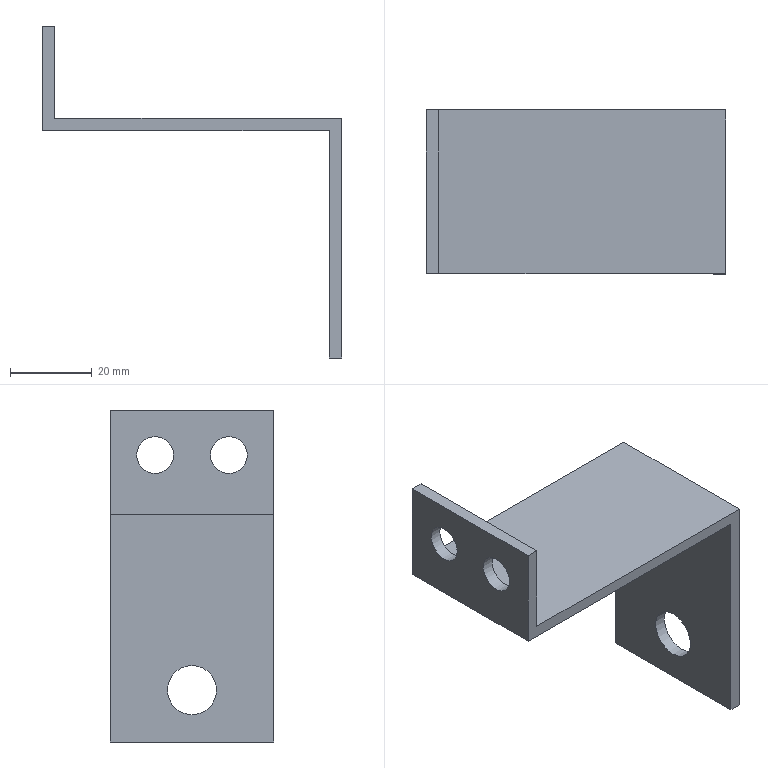Part | NX | features 1605242049 2 | 1 solid | 13 faces | box 73 x 40 x 81.051 mm | volume 17405 mm3 | plane 10 | cylinder 3 | commonest cylinder face diameters 9 x2 12 x1
STEP:
#1=CARTESIAN_POINT('',(1024.,-40.,36.449));
#2=VERTEX_POINT('',#1);
#3=CARTESIAN_POINT('',(1024.,-40.,-22.051));
#4=VERTEX_POINT('',#3);
#5=CARTESIAN_POINT('',(1024.,-40.,49.449));
#6=DIRECTION('',(0.,0.,1.));
#7=VECTOR('',#6,1000.);
#8=LINE('',#5,#7);
#9=EDGE_CURVE('',#2,#4,#8,.F.);
#10=ORIENTED_EDGE('',*,*,#9,.T.);
#11=CARTESIAN_POINT('',(1021.,-40.,-22.051));
#12=VERTEX_POINT('',#11);
#13=CARTESIAN_POINT('',(1047.,-40.,-22.051));
#14=DIRECTION('',(-1.,0.,0.));
#15=VECTOR('',#14,1000.);
#16=LINE('',#13,#15);
#17=EDGE_CURVE('',#12,#4,#16,.F.);
#18=ORIENTED_EDGE('',*,*,#17,.F.);
#19=CARTESIAN_POINT('',(1021.,-40.,33.449));
#20=VERTEX_POINT('',#19);
#21=CARTESIAN_POINT('',(1021.,-40.,6.449));
#22=DIRECTION('',(0.,0.,1.));
#23=VECTOR('',#22,1000.);
#24=LINE('',#21,#23);
#25=EDGE_CURVE('',#20,#12,#24,.F.);
#26=ORIENTED_EDGE('',*,*,#25,.F.);
#27=CARTESIAN_POINT('',(951.,-40.,33.449));
#28=VERTEX_POINT('',#27);
#29=CARTESIAN_POINT('',(973.,-40.,33.449));
#30=DIRECTION('',(-1.,0.,0.));
#31=VECTOR('',#30,1000.);
#32=LINE('',#29,#31);
#33=EDGE_CURVE('',#28,#20,#32,.F.);
#34=ORIENTED_EDGE('',*,*,#33,.F.);
#35=CARTESIAN_POINT('',(951.,-40.,59.));
#36=VERTEX_POINT('',#35);
#37=CARTESIAN_POINT('',(951.,-40.,49.449));
#38=DIRECTION('',(0.,0.,1.));
#39=VECTOR('',#38,1000.);
#40=LINE('',#37,#39);
#41=EDGE_CURVE('',#36,#28,#40,.F.);
#42=ORIENTED_EDGE('',*,*,#41,.F.);
#43=CARTESIAN_POINT('',(954.,-40.,59.));
#44=VERTEX_POINT('',#43);
#45=CARTESIAN_POINT('',(938.5,-40.,59.));
#46=DIRECTION('',(1.,0.,0.));
#47=VECTOR('',#46,1000.);
#48=LINE('',#45,#47);
#49=EDGE_CURVE('',#44,#36,#48,.F.);
#50=ORIENTED_EDGE('',*,*,#49,.F.);
#51=CARTESIAN_POINT('',(954.,-40.,36.449));
#52=VERTEX_POINT('',#51);
#53=CARTESIAN_POINT('',(954.,-40.,49.449));
#54=DIRECTION('',(0.,0.,1.));
#55=VECTOR('',#54,1000.);
#56=LINE('',#53,#55);
#57=EDGE_CURVE('',#44,#52,#56,.F.);
#58=ORIENTED_EDGE('',*,*,#57,.T.);
#59=CARTESIAN_POINT('',(973.,-40.,36.449));
#60=DIRECTION('',(-1.,0.,0.));
#61=VECTOR('',#60,1000.);
#62=LINE('',#59,#61);
#63=EDGE_CURVE('',#52,#2,#62,.F.);
#64=ORIENTED_EDGE('',*,*,#63,.T.);
#65=EDGE_LOOP('',(#10,#18,#26,#34,#42,#50,#58,#64));
#66=FACE_BOUND('',#65,.T.);
#67=CARTESIAN_POINT('',(973.,-40.,49.449));
#68=DIRECTION('',(0.,1.,0.));
#69=DIRECTION('',(1.,0.,0.));
#70=AXIS2_PLACEMENT_3D('',#67,#68,#69);
#71=PLANE('',#70);
#72=ADVANCED_FACE('',(#66),#71,.T.);
#73=CARTESIAN_POINT('',(1021.,-80.,-22.051));
#74=VERTEX_POINT('',#73);
#75=CARTESIAN_POINT('',(1021.,-80.,33.449));
#76=VERTEX_POINT('',#75);
#77=CARTESIAN_POINT('',(1021.,-80.,6.449));
#78=DIRECTION('',(0.,0.,-1.));
#79=VECTOR('',#78,1000.);
#80=LINE('',#77,#79);
#81=EDGE_CURVE('',#74,#76,#80,.F.);
#82=ORIENTED_EDGE('',*,*,#81,.F.);
#83=CARTESIAN_POINT('',(1024.,-80.,-22.051));
#84=VERTEX_POINT('',#83);
#85=CARTESIAN_POINT('',(1047.,-80.,-22.051));
#86=DIRECTION('',(1.,0.,0.));
#87=VECTOR('',#86,1000.);
#88=LINE('',#85,#87);
#89=EDGE_CURVE('',#84,#74,#88,.F.);
#90=ORIENTED_EDGE('',*,*,#89,.F.);
#91=CARTESIAN_POINT('',(1024.,-80.,36.449));
#92=VERTEX_POINT('',#91);
#93=CARTESIAN_POINT('',(1024.,-80.,49.449));
#94=DIRECTION('',(0.,0.,-1.));
#95=VECTOR('',#94,1000.);
#96=LINE('',#93,#95);
#97=EDGE_CURVE('',#84,#92,#96,.F.);
#98=ORIENTED_EDGE('',*,*,#97,.T.);
#99=CARTESIAN_POINT('',(954.,-80.,36.449));
#100=VERTEX_POINT('',#99);
#101=CARTESIAN_POINT('',(973.,-80.,36.449));
#102=DIRECTION('',(1.,0.,0.));
#103=VECTOR('',#102,1000.);
#104=LINE('',#101,#103);
#105=EDGE_CURVE('',#92,#100,#104,.F.);
#106=ORIENTED_EDGE('',*,*,#105,.T.);
#107=CARTESIAN_POINT('',(954.,-80.,59.));
#108=VERTEX_POINT('',#107);
#109=CARTESIAN_POINT('',(954.,-80.,49.449));
#110=DIRECTION('',(0.,0.,-1.));
#111=VECTOR('',#110,1000.);
#112=LINE('',#109,#111);
#113=EDGE_CURVE('',#100,#108,#112,.F.);
#114=ORIENTED_EDGE('',*,*,#113,.T.);
#115=CARTESIAN_POINT('',(951.,-80.,59.));
#116=VERTEX_POINT('',#115);
#117=CARTESIAN_POINT('',(938.5,-80.,59.));
#118=DIRECTION('',(-1.,0.,0.));
#119=VECTOR('',#118,1000.);
#120=LINE('',#117,#119);
#121=EDGE_CURVE('',#116,#108,#120,.F.);
#122=ORIENTED_EDGE('',*,*,#121,.F.);
#123=CARTESIAN_POINT('',(951.,-80.,33.449));
#124=VERTEX_POINT('',#123);
#125=CARTESIAN_POINT('',(951.,-80.,49.449));
#126=DIRECTION('',(0.,0.,-1.));
#127=VECTOR('',#126,1000.);
#128=LINE('',#125,#127);
#129=EDGE_CURVE('',#124,#116,#128,.F.);
#130=ORIENTED_EDGE('',*,*,#129,.F.);
#131=CARTESIAN_POINT('',(973.,-80.,33.449));
#132=DIRECTION('',(1.,0.,0.));
#133=VECTOR('',#132,1000.);
#134=LINE('',#131,#133);
#135=EDGE_CURVE('',#76,#124,#134,.F.);
#136=ORIENTED_EDGE('',*,*,#135,.F.);
#137=EDGE_LOOP('',(#82,#90,#98,#106,#114,#122,#130,#136));
#138=FACE_BOUND('',#137,.T.);
#139=CARTESIAN_POINT('',(973.,-80.,49.449));
#140=DIRECTION('',(0.,-1.,0.));
#141=DIRECTION('',(-1.,0.,0.));
#142=AXIS2_PLACEMENT_3D('',#139,#140,#141);
#143=PLANE('',#142);
#144=ADVANCED_FACE('',(#138),#143,.T.);
#145=CARTESIAN_POINT('',(951.,-64.5,48.));
#146=VERTEX_POINT('',#145);
#147=CARTESIAN_POINT('',(951.,-69.,48.));
#148=DIRECTION('',(1.,0.,0.));
#149=DIRECTION('',(0.,1.,0.));
#150=AXIS2_PLACEMENT_3D('',#147,#148,#149);
#151=CIRCLE('',#150,4.5);
#152=EDGE_CURVE('',#146,#146,#151,.F.);
#153=ORIENTED_EDGE('',*,*,#152,.T.);
#154=EDGE_LOOP('',(#153));
#155=FACE_BOUND('',#154,.T.);
#156=CARTESIAN_POINT('',(954.,-64.5,48.));
#157=VERTEX_POINT('',#156);
#158=CARTESIAN_POINT('',(954.,-69.,48.));
#159=DIRECTION('',(1.,0.,0.));
#160=DIRECTION('',(0.,1.,0.));
#161=AXIS2_PLACEMENT_3D('',#158,#159,#160);
#162=CIRCLE('',#161,4.5);
#163=EDGE_CURVE('',#157,#157,#162,.F.);
#164=ORIENTED_EDGE('',*,*,#163,.F.);
#165=EDGE_LOOP('',(#164));
#166=FACE_BOUND('',#165,.T.);
#167=CARTESIAN_POINT('',(954.,-69.,48.));
#168=DIRECTION('',(-1.,0.,0.));
#169=DIRECTION('',(0.,0.,-1.));
#170=AXIS2_PLACEMENT_3D('',#167,#168,#169);
#171=CYLINDRICAL_SURFACE('',#170,4.5);
#172=ADVANCED_FACE('',(#155,#166),#171,.F.);
#173=ORIENTED_EDGE('',*,*,#9,.F.);
#174=CARTESIAN_POINT('',(1024.,-82.,36.449));
#175=DIRECTION('',(0.,-1.,0.));
#176=VECTOR('',#175,1000.);
#177=LINE('',#174,#176);
#178=EDGE_CURVE('',#92,#2,#177,.F.);
#179=ORIENTED_EDGE('',*,*,#178,.F.);
#180=ORIENTED_EDGE('',*,*,#97,.F.);
#181=CARTESIAN_POINT('',(1024.,-82.,-22.051));
#182=DIRECTION('',(0.,-1.,0.));
#183=VECTOR('',#182,1000.);
#184=LINE('',#181,#183);
#185=EDGE_CURVE('',#84,#4,#184,.F.);
#186=ORIENTED_EDGE('',*,*,#185,.T.);
#187=EDGE_LOOP('',(#173,#179,#180,#186));
#188=FACE_BOUND('',#187,.T.);
#189=CARTESIAN_POINT('',(1024.,-60.,-15.384));
#190=VERTEX_POINT('',#189);
#191=CARTESIAN_POINT('',(1024.,-60.,-9.384));
#192=DIRECTION('',(1.,0.,0.));
#193=DIRECTION('',(0.,0.,-1.));
#194=AXIS2_PLACEMENT_3D('',#191,#192,#193);
#195=CIRCLE('',#194,6.);
#196=EDGE_CURVE('',#190,#190,#195,.F.);
#197=ORIENTED_EDGE('',*,*,#196,.T.);
#198=EDGE_LOOP('',(#197));
#199=FACE_BOUND('',#198,.T.);
#200=CARTESIAN_POINT('',(1024.,-82.,9.949));
#201=DIRECTION('',(-1.,0.,0.));
#202=DIRECTION('',(0.,1.,0.));
#203=AXIS2_PLACEMENT_3D('',#200,#201,#202);
#204=PLANE('',#203);
#205=ADVANCED_FACE('',(#188,#199),#204,.F.);
#206=ORIENTED_EDGE('',*,*,#81,.T.);
#207=CARTESIAN_POINT('',(1021.,-82.,33.449));
#208=DIRECTION('',(0.,-1.,0.));
#209=VECTOR('',#208,1000.);
#210=LINE('',#207,#209);
#211=EDGE_CURVE('',#76,#20,#210,.F.);
#212=ORIENTED_EDGE('',*,*,#211,.T.);
#213=ORIENTED_EDGE('',*,*,#25,.T.);
#214=CARTESIAN_POINT('',(1021.,-82.,-22.051));
#215=DIRECTION('',(0.,-1.,0.));
#216=VECTOR('',#215,1000.);
#217=LINE('',#214,#216);
#218=EDGE_CURVE('',#74,#12,#217,.F.);
#219=ORIENTED_EDGE('',*,*,#218,.F.);
#220=EDGE_LOOP('',(#206,#212,#213,#219));
#221=FACE_BOUND('',#220,.T.);
#222=CARTESIAN_POINT('',(1021.,-60.,-15.384));
#223=VERTEX_POINT('',#222);
#224=CARTESIAN_POINT('',(1021.,-60.,-9.384));
#225=DIRECTION('',(1.,0.,0.));
#226=DIRECTION('',(0.,0.,-1.));
#227=AXIS2_PLACEMENT_3D('',#224,#225,#226);
#228=CIRCLE('',#227,6.);
#229=EDGE_CURVE('',#223,#223,#228,.F.);
#230=ORIENTED_EDGE('',*,*,#229,.F.);
#231=EDGE_LOOP('',(#230));
#232=FACE_BOUND('',#231,.T.);
#233=CARTESIAN_POINT('',(1021.,-82.,6.449));
#234=DIRECTION('',(-1.,0.,0.));
#235=DIRECTION('',(0.,1.,0.));
#236=AXIS2_PLACEMENT_3D('',#233,#234,#235);
#237=PLANE('',#236);
#238=ADVANCED_FACE('',(#221,#232),#237,.T.);
#239=ORIENTED_EDGE('',*,*,#211,.F.);
#240=ORIENTED_EDGE('',*,*,#135,.T.);
#241=CARTESIAN_POINT('',(951.,-82.,33.449));
#242=DIRECTION('',(0.,-1.,0.));
#243=VECTOR('',#242,1000.);
#244=LINE('',#241,#243);
#245=EDGE_CURVE('',#124,#28,#244,.F.);
#246=ORIENTED_EDGE('',*,*,#245,.T.);
#247=ORIENTED_EDGE('',*,*,#33,.T.);
#248=EDGE_LOOP('',(#239,#240,#246,#247));
#249=FACE_BOUND('',#248,.T.);
#250=CARTESIAN_POINT('',(973.,-82.,33.449));
#251=DIRECTION('',(0.,0.,-1.));
#252=DIRECTION('',(0.,1.,0.));
#253=AXIS2_PLACEMENT_3D('',#250,#251,#252);
#254=PLANE('',#253);
#255=ADVANCED_FACE('',(#249),#254,.T.);
#256=CARTESIAN_POINT('',(954.,-82.,36.449));
#257=DIRECTION('',(0.,-1.,0.));
#258=VECTOR('',#257,1000.);
#259=LINE('',#256,#258);
#260=EDGE_CURVE('',#100,#52,#259,.F.);
#261=ORIENTED_EDGE('',*,*,#260,.F.);
#262=ORIENTED_EDGE('',*,*,#105,.F.);
#263=ORIENTED_EDGE('',*,*,#178,.T.);
#264=ORIENTED_EDGE('',*,*,#63,.F.);
#265=EDGE_LOOP('',(#261,#262,#263,#264));
#266=FACE_BOUND('',#265,.T.);
#267=CARTESIAN_POINT('',(973.,-82.,36.449));
#268=DIRECTION('',(0.,0.,-1.));
#269=DIRECTION('',(0.,1.,0.));
#270=AXIS2_PLACEMENT_3D('',#267,#268,#269);
#271=PLANE('',#270);
#272=ADVANCED_FACE('',(#266),#271,.F.);
#273=ORIENTED_EDGE('',*,*,#121,.T.);
#274=CARTESIAN_POINT('',(954.,-82.,59.));
#275=DIRECTION('',(0.,-1.,0.));
#276=VECTOR('',#275,1000.);
#277=LINE('',#274,#276);
#278=EDGE_CURVE('',#108,#44,#277,.F.);
#279=ORIENTED_EDGE('',*,*,#278,.T.);
#280=ORIENTED_EDGE('',*,*,#49,.T.);
#281=CARTESIAN_POINT('',(951.,-82.,59.));
#282=DIRECTION('',(0.,-1.,0.));
#283=VECTOR('',#282,1000.);
#284=LINE('',#281,#283);
#285=EDGE_CURVE('',#116,#36,#284,.F.);
#286=ORIENTED_EDGE('',*,*,#285,.F.);
#287=EDGE_LOOP('',(#273,#279,#280,#286));
#288=FACE_BOUND('',#287,.T.);
#289=CARTESIAN_POINT('',(938.5,-127.,59.));
#290=DIRECTION('',(0.,0.,-1.));
#291=DIRECTION('',(0.,1.,0.));
#292=AXIS2_PLACEMENT_3D('',#289,#290,#291);
#293=PLANE('',#292);
#294=ADVANCED_FACE('',(#288),#293,.F.);
#295=CARTESIAN_POINT('',(951.,-46.5,48.));
#296=VERTEX_POINT('',#295);
#297=CARTESIAN_POINT('',(951.,-51.,48.));
#298=DIRECTION('',(1.,0.,0.));
#299=DIRECTION('',(0.,1.,0.));
#300=AXIS2_PLACEMENT_3D('',#297,#298,#299);
#301=CIRCLE('',#300,4.5);
#302=EDGE_CURVE('',#296,#296,#301,.F.);
#303=ORIENTED_EDGE('',*,*,#302,.T.);
#304=EDGE_LOOP('',(#303));
#305=FACE_BOUND('',#304,.T.);
#306=CARTESIAN_POINT('',(954.,-46.5,48.));
#307=VERTEX_POINT('',#306);
#308=CARTESIAN_POINT('',(954.,-51.,48.));
#309=DIRECTION('',(1.,0.,0.));
#310=DIRECTION('',(0.,1.,0.));
#311=AXIS2_PLACEMENT_3D('',#308,#309,#310);
#312=CIRCLE('',#311,4.5);
#313=EDGE_CURVE('',#307,#307,#312,.F.);
#314=ORIENTED_EDGE('',*,*,#313,.F.);
#315=EDGE_LOOP('',(#314));
#316=FACE_BOUND('',#315,.T.);
#317=CARTESIAN_POINT('',(954.,-51.,48.));
#318=DIRECTION('',(-1.,0.,0.));
#319=DIRECTION('',(0.,0.,-1.));
#320=AXIS2_PLACEMENT_3D('',#317,#318,#319);
#321=CYLINDRICAL_SURFACE('',#320,4.5);
#322=ADVANCED_FACE('',(#305,#316),#321,.F.);
#323=ORIENTED_EDGE('',*,*,#163,.T.);
#324=EDGE_LOOP('',(#323));
#325=FACE_BOUND('',#324,.T.);
#326=ORIENTED_EDGE('',*,*,#313,.T.);
#327=EDGE_LOOP('',(#326));
#328=FACE_BOUND('',#327,.T.);
#329=ORIENTED_EDGE('',*,*,#278,.F.);
#330=ORIENTED_EDGE('',*,*,#113,.F.);
#331=ORIENTED_EDGE('',*,*,#260,.T.);
#332=ORIENTED_EDGE('',*,*,#57,.F.);
#333=EDGE_LOOP('',(#329,#330,#331,#332));
#334=FACE_BOUND('',#333,.T.);
#335=CARTESIAN_POINT('',(954.,-82.,49.449));
#336=DIRECTION('',(-1.,0.,0.));
#337=DIRECTION('',(0.,1.,0.));
#338=AXIS2_PLACEMENT_3D('',#335,#336,#337);
#339=PLANE('',#338);
#340=ADVANCED_FACE('',(#325,#328,#334),#339,.F.);
#341=ORIENTED_EDGE('',*,*,#152,.F.);
#342=EDGE_LOOP('',(#341));
#343=FACE_BOUND('',#342,.T.);
#344=ORIENTED_EDGE('',*,*,#302,.F.);
#345=EDGE_LOOP('',(#344));
#346=FACE_BOUND('',#345,.T.);
#347=ORIENTED_EDGE('',*,*,#285,.T.);
#348=ORIENTED_EDGE('',*,*,#41,.T.);
#349=ORIENTED_EDGE('',*,*,#245,.F.);
#350=ORIENTED_EDGE('',*,*,#129,.T.);
#351=EDGE_LOOP('',(#347,#348,#349,#350));
#352=FACE_BOUND('',#351,.T.);
#353=CARTESIAN_POINT('',(951.,-82.,49.449));
#354=DIRECTION('',(-1.,0.,0.));
#355=DIRECTION('',(0.,0.,-1.));
#356=AXIS2_PLACEMENT_3D('',#353,#354,#355);
#357=PLANE('',#356);
#358=ADVANCED_FACE('',(#343,#346,#352),#357,.T.);
#359=ORIENTED_EDGE('',*,*,#229,.T.);
#360=EDGE_LOOP('',(#359));
#361=FACE_BOUND('',#360,.T.);
#362=ORIENTED_EDGE('',*,*,#196,.F.);
#363=EDGE_LOOP('',(#362));
#364=FACE_BOUND('',#363,.T.);
#365=CARTESIAN_POINT('',(1041.468,-60.,-9.384));
#366=DIRECTION('',(1.,0.,-0.000000009));
#367=DIRECTION('',(0.000000009,0.,1.));
#368=AXIS2_PLACEMENT_3D('',#365,#366,#367);
#369=CYLINDRICAL_SURFACE('',#368,6.);
#370=ADVANCED_FACE('',(#361,#364),#369,.F.);
#371=ORIENTED_EDGE('',*,*,#17,.T.);
#372=ORIENTED_EDGE('',*,*,#185,.F.);
#373=ORIENTED_EDGE('',*,*,#89,.T.);
#374=ORIENTED_EDGE('',*,*,#218,.T.);
#375=EDGE_LOOP('',(#371,#372,#373,#374));
#376=FACE_BOUND('',#375,.T.);
#377=CARTESIAN_POINT('',(1047.,-82.,-22.051));
#378=DIRECTION('',(0.,0.,-1.));
#379=DIRECTION('',(1.,0.,0.));
#380=AXIS2_PLACEMENT_3D('',#377,#378,#379);
#381=PLANE('',#380);
#382=ADVANCED_FACE('',(#376),#381,.T.);
#383=CLOSED_SHELL('',(#72,#144,#172,#205,#238,#255,#272,#294,#322,#340,#358,#370,#382));
#384=MANIFOLD_SOLID_BREP('',#383);
#385=(LENGTH_UNIT()NAMED_UNIT(*)SI_UNIT(.MILLI.,.METRE.));
#386=UNCERTAINTY_MEASURE_WITH_UNIT(LENGTH_MEASURE(0.00001),#385,'','');
#387=(NAMED_UNIT(*)PLANE_ANGLE_UNIT()SI_UNIT($,.RADIAN.));
#388=(NAMED_UNIT(*)SI_UNIT($,.STERADIAN.)SOLID_ANGLE_UNIT());
#389=(GEOMETRIC_REPRESENTATION_CONTEXT(3)GLOBAL_UNCERTAINTY_ASSIGNED_CONTEXT((#386))GLOBAL_UNIT_ASSIGNED_CONTEXT((#385,#387,#388))REPRESENTATION_CONTEXT('',''));
#390=ADVANCED_BREP_SHAPE_REPRESENTATION('',(#384),#389);